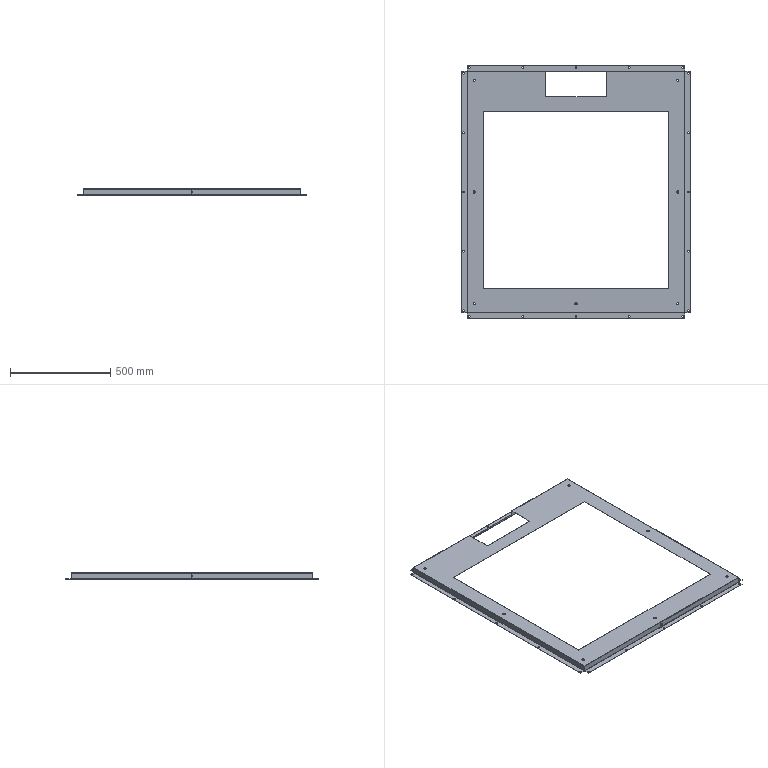Part | SolidWorks | features ICE 7, EdgeFlange 2, FlatPattern 1, SMBaseFlange 1, SheetMetal 1 | 1 solid | 194 faces | box 1139 x 1259 x 30 mm | volume 692290 mm3 | plane 98 | cylinder 88 | spline 8 | commonest cylinder face diameters 7 x50 11 x14 0.4 x9 2.4 x9 10 x6